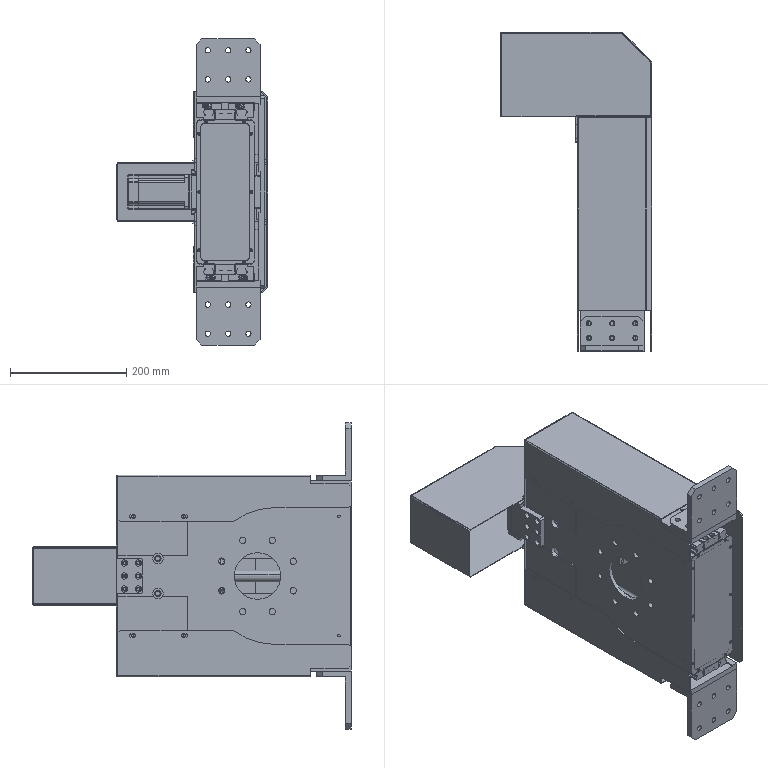Part | SolidWorks | features InContextFeatHolder 2 | 107 solids | 9774 faces | volume 6265247 mm3 | plane 5250 | cylinder 3182 | cone 651 | spline 560 | torus 83 | sphere 48 | commonest cylinder face diameters 1 x648 0.2 x272 2 x246 4.06 x176 6 x147 0.1 x144